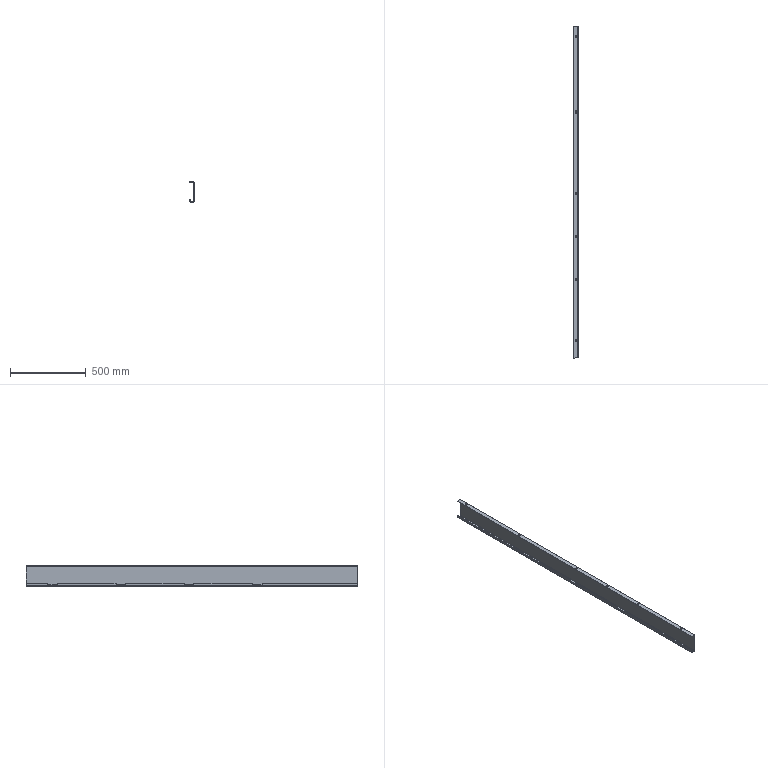Part | NX | features solid 2 | 1 solid | 83 faces | box 28 x 2189 x 132 mm | volume 859020 mm3 | plane 65 | cylinder 18 | commonest cylinder face diameters 10 x12 2 x3 6 x3